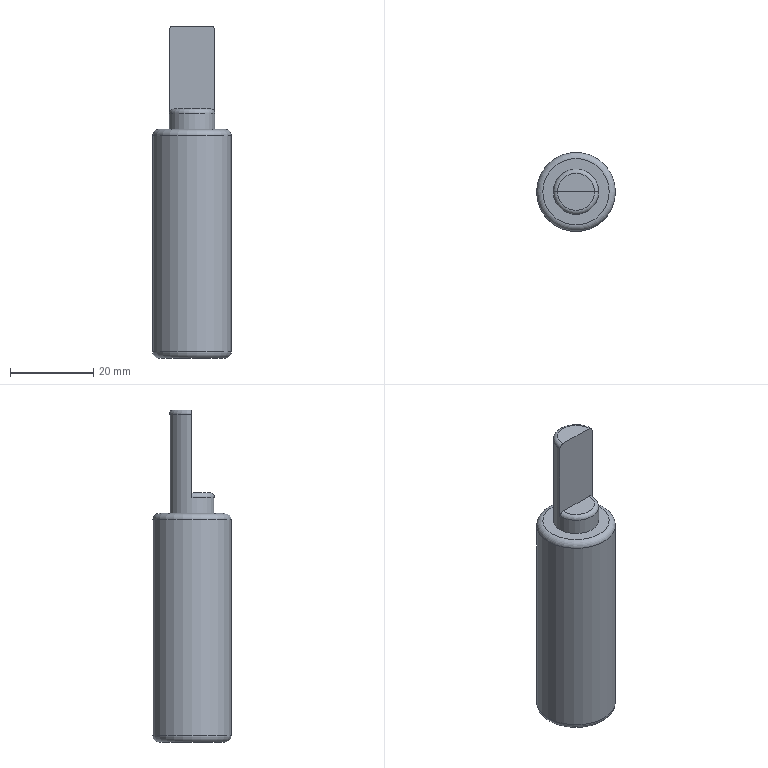Part | STEP file | 1_id1178_x_t | 1 solid | 13 faces | box 19 x 19 x 80 mm | volume 16778 mm3 | plane 5 | torus 4 | cylinder 3 | cone 1 | commonest cylinder face diameters 5.156 x1 10.922 x1 19 x1
STEP:
#1=CARTESIAN_POINT('',(0.,0.,0.));
#2=DIRECTION('',(0.,0.,1.));
#3=DIRECTION('',(1.,0.,0.));
#4=AXIS2_PLACEMENT_3D('',#1,#2,#3);
#5=CARTESIAN_POINT('',(687.464,177.5,-76.53));
#6=VERTEX_POINT('',#5);
#7=CARTESIAN_POINT('',(688.464,177.5,-75.53));
#8=VERTEX_POINT('',#7);
#9=CARTESIAN_POINT('',(687.464,177.5,-76.53));
#10=CARTESIAN_POINT('',(687.464,177.5,-76.418));
#11=CARTESIAN_POINT('',(687.483,177.5,-76.305));
#12=CARTESIAN_POINT('',(687.52,177.5,-76.199));
#13=CARTESIAN_POINT('',(687.557,177.5,-76.093));
#14=CARTESIAN_POINT('',(687.613,177.5,-75.993));
#15=CARTESIAN_POINT('',(687.683,177.5,-75.905));
#16=CARTESIAN_POINT('',(687.753,177.5,-75.818));
#17=CARTESIAN_POINT('',(687.839,177.5,-75.741));
#18=CARTESIAN_POINT('',(687.934,177.5,-75.682));
#19=CARTESIAN_POINT('',(688.029,177.5,-75.623));
#20=CARTESIAN_POINT('',(688.135,177.5,-75.579));
#21=CARTESIAN_POINT('',(688.244,177.5,-75.554));
#22=CARTESIAN_POINT('',(688.316,177.5,-75.538));
#23=CARTESIAN_POINT('',(688.39,177.5,-75.53));
#24=CARTESIAN_POINT('',(688.464,177.5,-75.53));
#25=B_SPLINE_CURVE_WITH_KNOTS('',3,(#9,#10,#11,#12,#13,#14,#15,#16,#17,#18,#19,#20,#21,#22,#23,#24),.UNSPECIFIED.,.F.,.F.,(4,3,3,3,3,4),(0.,0.2149,0.4299,0.6448,0.8598,1.),.UNSPECIFIED.);
#26=CARTESIAN_POINT('',(351.838,177.5,-123.402));
#27=DIRECTION('',(0.,1.,0.));
#28=DIRECTION('',(0.,0.,-1.));
#29=AXIS2_PLACEMENT_3D('',#26,#27,#28);
#30=PLANE('',#29);
#31=CARTESIAN_POINT('',(-46.872,-335.625));
#32=CARTESIAN_POINT('',(-46.984,-335.625));
#33=CARTESIAN_POINT('',(-47.098,-335.645));
#34=CARTESIAN_POINT('',(-47.203,-335.682));
#35=CARTESIAN_POINT('',(-47.309,-335.719));
#36=CARTESIAN_POINT('',(-47.409,-335.775));
#37=CARTESIAN_POINT('',(-47.497,-335.845));
#38=CARTESIAN_POINT('',(-47.584,-335.914));
#39=CARTESIAN_POINT('',(-47.661,-336.));
#40=CARTESIAN_POINT('',(-47.72,-336.095));
#41=CARTESIAN_POINT('',(-47.779,-336.19));
#42=CARTESIAN_POINT('',(-47.823,-336.297));
#43=CARTESIAN_POINT('',(-47.848,-336.406));
#44=CARTESIAN_POINT('',(-47.864,-336.478));
#45=CARTESIAN_POINT('',(-47.872,-336.552));
#46=CARTESIAN_POINT('',(-47.872,-336.625));
#47=B_SPLINE_CURVE_WITH_KNOTS('',3,(#31,#32,#33,#34,#35,#36,#37,#38,#39,#40,#41,#42,#43,#44,#45,#46),.UNSPECIFIED.,.F.,.F.,(4,3,3,3,3,4),(0.,0.2149,0.4299,0.6448,0.8598,1.),.UNSPECIFIED.);
#48=(GEOMETRIC_REPRESENTATION_CONTEXT(2)PARAMETRIC_REPRESENTATION_CONTEXT()REPRESENTATION_CONTEXT('',''));
#49=DEFINITIONAL_REPRESENTATION('',(#47),#48);
#50=PCURVE('',#30,#49);
#51=CARTESIAN_POINT('',(692.925,177.5,-76.53));
#52=DIRECTION('',(0.,0.,1.));
#53=DIRECTION('',(1.,0.,0.));
#54=AXIS2_PLACEMENT_3D('',#51,#52,#53);
#55=TOROIDAL_SURFACE('',#54,4.461,1.);
#56=CARTESIAN_POINT('',(3.142,0.));
#57=CARTESIAN_POINT('',(3.142,1.571));
#58=B_SPLINE_CURVE_WITH_KNOTS('',1,(#56,#57),.UNSPECIFIED.,.F.,.F.,(2,2),(0.,1.),.PIECEWISE_BEZIER_KNOTS.);
#59=(GEOMETRIC_REPRESENTATION_CONTEXT(2)PARAMETRIC_REPRESENTATION_CONTEXT()REPRESENTATION_CONTEXT('',''));
#60=DEFINITIONAL_REPRESENTATION('',(#58),#59);
#61=PCURVE('',#55,#60);
#62=SURFACE_CURVE('',#25,(#50,#61),.PCURVE_S1.);
#63=EDGE_CURVE('',#6,#8,#62,.T.);
#64=ORIENTED_EDGE('',*,*,#63,.F.);
#65=CARTESIAN_POINT('',(687.464,177.5,-56.53));
#66=VERTEX_POINT('',#65);
#67=CARTESIAN_POINT('',(687.464,177.5,-123.402));
#68=DIRECTION('',(0.,0.,1.));
#69=VECTOR('',#68,1.);
#70=LINE('',#67,#69);
#71=CARTESIAN_POINT('',(0.,-335.625));
#72=DIRECTION('',(-1.,0.));
#73=VECTOR('',#72,1.);
#74=LINE('',#71,#73);
#75=(GEOMETRIC_REPRESENTATION_CONTEXT(2)PARAMETRIC_REPRESENTATION_CONTEXT()REPRESENTATION_CONTEXT('',''));
#76=DEFINITIONAL_REPRESENTATION('',(#74),#75);
#77=PCURVE('',#30,#76);
#78=CARTESIAN_POINT('',(692.925,177.5,-142.23));
#79=DIRECTION('',(0.,0.,1.));
#80=DIRECTION('',(-1.,0.,0.));
#81=AXIS2_PLACEMENT_3D('',#78,#79,#80);
#82=CYLINDRICAL_SURFACE('',#81,5.461);
#83=CARTESIAN_POINT('',(6.283,18.828));
#84=DIRECTION('',(0.,1.));
#85=VECTOR('',#84,1.);
#86=LINE('',#83,#85);
#87=(GEOMETRIC_REPRESENTATION_CONTEXT(2)PARAMETRIC_REPRESENTATION_CONTEXT()REPRESENTATION_CONTEXT('',''));
#88=DEFINITIONAL_REPRESENTATION('',(#86),#87);
#89=PCURVE('',#82,#88);
#90=SURFACE_CURVE('',#70,(#77,#89),.PCURVE_S1.);
#91=EDGE_CURVE('',#6,#66,#90,.T.);
#92=ORIENTED_EDGE('',*,*,#91,.T.);
#93=CARTESIAN_POINT('',(688.464,177.5,-55.53));
#94=VERTEX_POINT('',#93);
#95=CARTESIAN_POINT('',(688.464,177.5,-55.53));
#96=CARTESIAN_POINT('',(688.352,177.5,-55.53));
#97=CARTESIAN_POINT('',(688.238,177.5,-55.549));
#98=CARTESIAN_POINT('',(688.133,177.5,-55.586));
#99=CARTESIAN_POINT('',(688.027,177.5,-55.623));
#100=CARTESIAN_POINT('',(687.927,177.5,-55.679));
#101=CARTESIAN_POINT('',(687.839,177.5,-55.749));
#102=CARTESIAN_POINT('',(687.752,177.5,-55.819));
#103=CARTESIAN_POINT('',(687.675,177.5,-55.905));
#104=CARTESIAN_POINT('',(687.616,177.5,-56.));
#105=CARTESIAN_POINT('',(687.557,177.5,-56.095));
#106=CARTESIAN_POINT('',(687.513,177.5,-56.201));
#107=CARTESIAN_POINT('',(687.488,177.5,-56.31));
#108=CARTESIAN_POINT('',(687.472,177.5,-56.382));
#109=CARTESIAN_POINT('',(687.464,177.5,-56.456));
#110=CARTESIAN_POINT('',(687.464,177.5,-56.53));
#111=B_SPLINE_CURVE_WITH_KNOTS('',3,(#95,#96,#97,#98,#99,#100,#101,#102,#103,#104,#105,#106,#107,#108,#109,#110),.UNSPECIFIED.,.F.,.F.,(4,3,3,3,3,4),(0.,0.2149,0.4299,0.6448,0.8598,1.),.UNSPECIFIED.);
#112=CARTESIAN_POINT('',(-67.872,-336.625));
#113=CARTESIAN_POINT('',(-67.872,-336.513));
#114=CARTESIAN_POINT('',(-67.853,-336.4));
#115=CARTESIAN_POINT('',(-67.816,-336.294));
#116=CARTESIAN_POINT('',(-67.779,-336.189));
#117=CARTESIAN_POINT('',(-67.723,-336.088));
#118=CARTESIAN_POINT('',(-67.653,-336.001));
#119=CARTESIAN_POINT('',(-67.583,-335.913));
#120=CARTESIAN_POINT('',(-67.497,-335.837));
#121=CARTESIAN_POINT('',(-67.402,-335.777));
#122=CARTESIAN_POINT('',(-67.307,-335.718));
#123=CARTESIAN_POINT('',(-67.201,-335.674));
#124=CARTESIAN_POINT('',(-67.092,-335.65));
#125=CARTESIAN_POINT('',(-67.02,-335.634));
#126=CARTESIAN_POINT('',(-66.946,-335.625));
#127=CARTESIAN_POINT('',(-66.872,-335.625));
#128=B_SPLINE_CURVE_WITH_KNOTS('',3,(#112,#113,#114,#115,#116,#117,#118,#119,#120,#121,#122,#123,#124,#125,#126,#127),.UNSPECIFIED.,.F.,.F.,(4,3,3,3,3,4),(0.,0.2149,0.4299,0.6448,0.8598,1.),.UNSPECIFIED.);
#129=(GEOMETRIC_REPRESENTATION_CONTEXT(2)PARAMETRIC_REPRESENTATION_CONTEXT()REPRESENTATION_CONTEXT('',''));
#130=DEFINITIONAL_REPRESENTATION('',(#128),#129);
#131=PCURVE('',#30,#130);
#132=CARTESIAN_POINT('',(692.925,177.5,-56.53));
#133=DIRECTION('',(0.,0.,1.));
#134=DIRECTION('',(1.,0.,0.));
#135=AXIS2_PLACEMENT_3D('',#132,#133,#134);
#136=TOROIDAL_SURFACE('',#135,4.461,1.);
#137=CARTESIAN_POINT('',(3.142,1.571));
#138=CARTESIAN_POINT('',(3.142,0.));
#139=B_SPLINE_CURVE_WITH_KNOTS('',1,(#137,#138),.UNSPECIFIED.,.F.,.F.,(2,2),(0.,1.),.PIECEWISE_BEZIER_KNOTS.);
#140=(GEOMETRIC_REPRESENTATION_CONTEXT(2)PARAMETRIC_REPRESENTATION_CONTEXT()REPRESENTATION_CONTEXT('',''));
#141=DEFINITIONAL_REPRESENTATION('',(#139),#140);
#142=PCURVE('',#136,#141);
#143=SURFACE_CURVE('',#111,(#131,#142),.PCURVE_S1.);
#144=EDGE_CURVE('',#94,#66,#143,.T.);
#145=ORIENTED_EDGE('',*,*,#144,.F.);
#146=CARTESIAN_POINT('',(697.386,177.5,-55.53));
#147=VERTEX_POINT('',#146);
#148=CARTESIAN_POINT('',(688.464,177.5,-55.53));
#149=DIRECTION('',(1.,0.000000541,0.));
#150=VECTOR('',#149,1.);
#151=LINE('',#148,#150);
#152=CARTESIAN_POINT('',(-67.872,-336.625));
#153=DIRECTION('',(0.,-1.));
#154=VECTOR('',#153,1.);
#155=LINE('',#152,#154);
#156=(GEOMETRIC_REPRESENTATION_CONTEXT(2)PARAMETRIC_REPRESENTATION_CONTEXT()REPRESENTATION_CONTEXT('',''));
#157=DEFINITIONAL_REPRESENTATION('',(#155),#156);
#158=PCURVE('',#30,#157);
#159=CARTESIAN_POINT('',(692.925,177.5,-55.53));
#160=DIRECTION('',(0.,0.,1.));
#161=DIRECTION('',(-1.,0.,0.));
#162=AXIS2_PLACEMENT_3D('',#159,#160,#161);
#163=PLANE('',#162);
#164=CARTESIAN_POINT('',(4.461,-0.00001102));
#165=DIRECTION('',(-1.,-0.000000541));
#166=VECTOR('',#165,1.);
#167=LINE('',#164,#166);
#168=(GEOMETRIC_REPRESENTATION_CONTEXT(2)PARAMETRIC_REPRESENTATION_CONTEXT()REPRESENTATION_CONTEXT('',''));
#169=DEFINITIONAL_REPRESENTATION('',(#167),#168);
#170=PCURVE('',#163,#169);
#171=SURFACE_CURVE('',#151,(#158,#170),.PCURVE_S1.);
#172=EDGE_CURVE('',#94,#147,#171,.T.);
#173=ORIENTED_EDGE('',*,*,#172,.T.);
#174=CARTESIAN_POINT('',(698.386,177.5,-56.53));
#175=VERTEX_POINT('',#174);
#176=CARTESIAN_POINT('',(697.386,177.5,-56.53));
#177=DIRECTION('',(0.000003245,-1.,0.));
#178=DIRECTION('',(1.,0.000003245,0.));
#179=AXIS2_PLACEMENT_3D('',#176,#177,#178);
#180=CIRCLE('',#179,1.);
#181=CARTESIAN_POINT('',(-66.872,-346.547));
#182=CARTESIAN_POINT('',(-68.604,-346.547));
#183=CARTESIAN_POINT('',(-67.738,-345.047));
#184=CARTESIAN_POINT('',(-66.872,-343.547));
#185=CARTESIAN_POINT('',(-66.006,-345.047));
#186=CARTESIAN_POINT('',(-65.14,-346.547));
#187=CARTESIAN_POINT('',(-66.872,-346.547));
#188=(BOUNDED_CURVE()B_SPLINE_CURVE(2,(#181,#182,#183,#184,#185,#186,#187),.UNSPECIFIED.,.T.,.F.)B_SPLINE_CURVE_WITH_KNOTS((1,2,2,2,2,1),(-2.094,0.,2.094,4.189,6.283,8.378),.UNSPECIFIED.)CURVE()GEOMETRIC_REPRESENTATION_ITEM()RATIONAL_B_SPLINE_CURVE((1.,0.5,1.,0.5,1.,0.5,1.))REPRESENTATION_ITEM(''));
#189=(GEOMETRIC_REPRESENTATION_CONTEXT(2)PARAMETRIC_REPRESENTATION_CONTEXT()REPRESENTATION_CONTEXT('',''));
#190=DEFINITIONAL_REPRESENTATION('',(#188),#189);
#191=PCURVE('',#30,#190);
#192=CARTESIAN_POINT('',(0.000003245,0.));
#193=DIRECTION('',(0.,1.));
#194=VECTOR('',#193,1.);
#195=LINE('',#192,#194);
#196=(GEOMETRIC_REPRESENTATION_CONTEXT(2)PARAMETRIC_REPRESENTATION_CONTEXT()REPRESENTATION_CONTEXT('',''));
#197=DEFINITIONAL_REPRESENTATION('',(#195),#196);
#198=PCURVE('',#136,#197);
#199=SURFACE_CURVE('',#180,(#191,#198),.PCURVE_S1.);
#200=EDGE_CURVE('',#175,#147,#199,.T.);
#201=ORIENTED_EDGE('',*,*,#200,.F.);
#202=CARTESIAN_POINT('',(698.386,177.5,-76.53));
#203=VERTEX_POINT('',#202);
#204=CARTESIAN_POINT('',(698.386,177.5,-76.53));
#205=DIRECTION('',(0.,-0.000000143,-1.));
#206=VECTOR('',#205,1.);
#207=LINE('',#204,#206);
#208=CARTESIAN_POINT('',(-46.872,-346.547));
#209=DIRECTION('',(1.,0.));
#210=VECTOR('',#209,1.);
#211=LINE('',#208,#210);
#212=(GEOMETRIC_REPRESENTATION_CONTEXT(2)PARAMETRIC_REPRESENTATION_CONTEXT()REPRESENTATION_CONTEXT('',''));
#213=DEFINITIONAL_REPRESENTATION('',(#211),#212);
#214=PCURVE('',#30,#213);
#215=CARTESIAN_POINT('',(3.142,65.7));
#216=DIRECTION('',(-0.000000026,-1.));
#217=VECTOR('',#216,1.);
#218=LINE('',#215,#217);
#219=(GEOMETRIC_REPRESENTATION_CONTEXT(2)PARAMETRIC_REPRESENTATION_CONTEXT()REPRESENTATION_CONTEXT('',''));
#220=DEFINITIONAL_REPRESENTATION('',(#218),#219);
#221=PCURVE('',#82,#220);
#222=SURFACE_CURVE('',#207,(#214,#221),.PCURVE_S1.);
#223=EDGE_CURVE('',#175,#203,#222,.T.);
#224=ORIENTED_EDGE('',*,*,#223,.T.);
#225=CARTESIAN_POINT('',(697.386,177.5,-75.53));
#226=VERTEX_POINT('',#225);
#227=CARTESIAN_POINT('',(697.386,177.5,-76.53));
#228=DIRECTION('',(-0.000003245,1.,0.));
#229=DIRECTION('',(0.,0.,1.));
#230=AXIS2_PLACEMENT_3D('',#227,#228,#229);
#231=CIRCLE('',#230,1.);
#232=CARTESIAN_POINT('',(-46.872,-345.547));
#233=DIRECTION('',(-1.,0.));
#234=AXIS2_PLACEMENT_2D('',#232,#233);
#235=CIRCLE('',#234,1.);
#236=(GEOMETRIC_REPRESENTATION_CONTEXT(2)PARAMETRIC_REPRESENTATION_CONTEXT()REPRESENTATION_CONTEXT('',''));
#237=DEFINITIONAL_REPRESENTATION('',(#235),#236);
#238=PCURVE('',#30,#237);
#239=CARTESIAN_POINT('',(6.283,1.571));
#240=DIRECTION('',(0.,-1.));
#241=VECTOR('',#240,1.);
#242=LINE('',#239,#241);
#243=(GEOMETRIC_REPRESENTATION_CONTEXT(2)PARAMETRIC_REPRESENTATION_CONTEXT()REPRESENTATION_CONTEXT('',''));
#244=DEFINITIONAL_REPRESENTATION('',(#242),#243);
#245=PCURVE('',#55,#244);
#246=SURFACE_CURVE('',#231,(#238,#245),.PCURVE_S1.);
#247=EDGE_CURVE('',#226,#203,#246,.T.);
#248=ORIENTED_EDGE('',*,*,#247,.F.);
#249=CARTESIAN_POINT('',(688.464,177.5,-75.53));
#250=DIRECTION('',(1.,0.000000541,0.));
#251=VECTOR('',#250,1.);
#252=LINE('',#249,#251);
#253=CARTESIAN_POINT('',(-47.872,-336.625));
#254=DIRECTION('',(0.,-1.));
#255=VECTOR('',#254,1.);
#256=LINE('',#253,#255);
#257=(GEOMETRIC_REPRESENTATION_CONTEXT(2)PARAMETRIC_REPRESENTATION_CONTEXT()REPRESENTATION_CONTEXT('',''));
#258=DEFINITIONAL_REPRESENTATION('',(#256),#257);
#259=PCURVE('',#30,#258);
#260=CARTESIAN_POINT('',(692.925,177.5,-75.53));
#261=DIRECTION('',(0.,0.,1.));
#262=DIRECTION('',(-1.,0.,0.));
#263=AXIS2_PLACEMENT_3D('',#260,#261,#262);
#264=PLANE('',#263);
#265=CARTESIAN_POINT('',(4.461,-0.00001102));
#266=DIRECTION('',(-1.,-0.000000541));
#267=VECTOR('',#266,1.);
#268=LINE('',#265,#267);
#269=(GEOMETRIC_REPRESENTATION_CONTEXT(2)PARAMETRIC_REPRESENTATION_CONTEXT()REPRESENTATION_CONTEXT('',''));
#270=DEFINITIONAL_REPRESENTATION('',(#268),#269);
#271=PCURVE('',#264,#270);
#272=SURFACE_CURVE('',#252,(#259,#271),.PCURVE_S1.);
#273=EDGE_CURVE('',#8,#226,#272,.T.);
#274=ORIENTED_EDGE('',*,*,#273,.F.);
#275=EDGE_LOOP('',(#64,#92,#145,#173,#201,#224,#248,#274));
#276=FACE_BOUND('',#275,.F.);
#277=ADVANCED_FACE('',(#276),#30,.F.);
#278=ORIENTED_EDGE('',*,*,#63,.F.);
#279=CARTESIAN_POINT('',(692.925,177.5,-76.53));
#280=DIRECTION('',(0.,0.,1.));
#281=DIRECTION('',(-1.,0.,0.));
#282=AXIS2_PLACEMENT_3D('',#279,#280,#281);
#283=CIRCLE('',#282,5.461);
#284=CARTESIAN_POINT('',(3.142,0.));
#285=DIRECTION('',(1.,0.));
#286=VECTOR('',#285,1.);
#287=LINE('',#284,#286);
#288=(GEOMETRIC_REPRESENTATION_CONTEXT(2)PARAMETRIC_REPRESENTATION_CONTEXT()REPRESENTATION_CONTEXT('',''));
#289=DEFINITIONAL_REPRESENTATION('',(#287),#288);
#290=PCURVE('',#55,#289);
#291=CARTESIAN_POINT('',(0.,65.7));
#292=DIRECTION('',(1.,0.));
#293=VECTOR('',#292,1.);
#294=LINE('',#291,#293);
#295=(GEOMETRIC_REPRESENTATION_CONTEXT(2)PARAMETRIC_REPRESENTATION_CONTEXT()REPRESENTATION_CONTEXT('',''));
#296=DEFINITIONAL_REPRESENTATION('',(#294),#295);
#297=PCURVE('',#82,#296);
#298=SURFACE_CURVE('',#283,(#290,#297),.PCURVE_S1.);
#299=EDGE_CURVE('',#6,#203,#298,.T.);
#300=ORIENTED_EDGE('',*,*,#299,.T.);
#301=ORIENTED_EDGE('',*,*,#247,.F.);
#302=CARTESIAN_POINT('',(692.925,177.5,-75.53));
#303=DIRECTION('',(0.,0.,1.));
#304=DIRECTION('',(-1.,0.000003705,0.));
#305=AXIS2_PLACEMENT_3D('',#302,#303,#304);
#306=CIRCLE('',#305,4.461);
#307=CARTESIAN_POINT('',(3.142,1.571));
#308=DIRECTION('',(1.,0.));
#309=VECTOR('',#308,1.);
#310=LINE('',#307,#309);
#311=(GEOMETRIC_REPRESENTATION_CONTEXT(2)PARAMETRIC_REPRESENTATION_CONTEXT()REPRESENTATION_CONTEXT('',''));
#312=DEFINITIONAL_REPRESENTATION('',(#310),#311);
#313=PCURVE('',#55,#312);
#314=CARTESIAN_POINT('',(0.,0.));
#315=DIRECTION('',(1.,-0.000003705));
#316=AXIS2_PLACEMENT_2D('',#314,#315);
#317=CIRCLE('',#316,4.461);
#318=(GEOMETRIC_REPRESENTATION_CONTEXT(2)PARAMETRIC_REPRESENTATION_CONTEXT()REPRESENTATION_CONTEXT('',''));
#319=DEFINITIONAL_REPRESENTATION('',(#317),#318);
#320=PCURVE('',#264,#319);
#321=SURFACE_CURVE('',#306,(#313,#320),.PCURVE_S1.);
#322=EDGE_CURVE('',#8,#226,#321,.T.);
#323=ORIENTED_EDGE('',*,*,#322,.F.);
#324=EDGE_LOOP('',(#278,#300,#301,#323));
#325=FACE_BOUND('',#324,.T.);
#326=ADVANCED_FACE('',(#325),#55,.T.);
#327=ORIENTED_EDGE('',*,*,#273,.F.);
#328=ORIENTED_EDGE('',*,*,#322,.T.);
#329=EDGE_LOOP('',(#327,#328));
#330=FACE_BOUND('',#329,.T.);
#331=ADVANCED_FACE('',(#330),#264,.T.);
#332=ORIENTED_EDGE('',*,*,#299,.F.);
#333=CARTESIAN_POINT('',(687.464,177.5,-80.457));
#334=VERTEX_POINT('',#333);
#335=CARTESIAN_POINT('',(687.464,177.5,-80.457));
#336=CARTESIAN_POINT('',(687.464,177.5,-76.53));
#337=B_SPLINE_CURVE_WITH_KNOTS('',1,(#335,#336),.UNSPECIFIED.,.F.,.F.,(2,2),(61.773,65.7),.PIECEWISE_BEZIER_KNOTS.);
#338=CARTESIAN_POINT('',(0.,0.));
#339=DIRECTION('',(0.,1.));
#340=VECTOR('',#339,1.);
#341=LINE('',#338,#340);
#342=(GEOMETRIC_REPRESENTATION_CONTEXT(2)PARAMETRIC_REPRESENTATION_CONTEXT()REPRESENTATION_CONTEXT('',''));
#343=DEFINITIONAL_REPRESENTATION('',(#341),#342);
#344=PCURVE('',#82,#343);
#345=CARTESIAN_POINT('',(6.283,0.));
#346=DIRECTION('',(0.,1.));
#347=VECTOR('',#346,1.);
#348=LINE('',#345,#347);
#349=(GEOMETRIC_REPRESENTATION_CONTEXT(2)PARAMETRIC_REPRESENTATION_CONTEXT()REPRESENTATION_CONTEXT('',''));
#350=DEFINITIONAL_REPRESENTATION('',(#348),#349);
#351=PCURVE('',#82,#350);
#352=SEAM_CURVE('',#337,(#344,#351),.PCURVE_S1.);
#353=EDGE_CURVE('',#334,#6,#352,.T.);
#354=ORIENTED_EDGE('',*,*,#353,.F.);
#355=CARTESIAN_POINT('',(698.386,177.5,-80.457));
#356=VERTEX_POINT('',#355);
#357=CARTESIAN_POINT('',(692.925,177.5,-80.457));
#358=DIRECTION('',(0.,0.,-1.));
#359=DIRECTION('',(1.,0.,0.));
#360=AXIS2_PLACEMENT_3D('',#357,#358,#359);
#361=CIRCLE('',#360,5.461);
#362=CARTESIAN_POINT('',(3.142,61.773));
#363=DIRECTION('',(-1.,0.));
#364=VECTOR('',#363,1.);
#365=LINE('',#362,#364);
#366=(GEOMETRIC_REPRESENTATION_CONTEXT(2)PARAMETRIC_REPRESENTATION_CONTEXT()REPRESENTATION_CONTEXT('',''));
#367=DEFINITIONAL_REPRESENTATION('',(#365),#366);
#368=PCURVE('',#82,#367);
#369=CARTESIAN_POINT('',(692.925,177.5,-80.457));
#370=DIRECTION('',(0.,0.,1.));
#371=DIRECTION('',(-1.,0.,0.));
#372=AXIS2_PLACEMENT_3D('',#369,#370,#371);
#373=PLANE('',#372);
#374=CARTESIAN_POINT('',(-5.461,0.));
#375=CARTESIAN_POINT('',(-5.461,9.459));
#376=CARTESIAN_POINT('',(2.731,4.729));
#377=CARTESIAN_POINT('',(10.922,0.));
#378=CARTESIAN_POINT('',(2.731,-4.729));
#379=CARTESIAN_POINT('',(-5.461,-9.459));
#380=CARTESIAN_POINT('',(-5.461,0.));
#381=(BOUNDED_CURVE()B_SPLINE_CURVE(2,(#374,#375,#376,#377,#378,#379,#380),.UNSPECIFIED.,.T.,.F.)B_SPLINE_CURVE_WITH_KNOTS((1,2,2,2,2,1),(-2.094,0.,2.094,4.189,6.283,8.378),.UNSPECIFIED.)CURVE()GEOMETRIC_REPRESENTATION_ITEM()RATIONAL_B_SPLINE_CURVE((1.,0.5,1.,0.5,1.,0.5,1.))REPRESENTATION_ITEM(''));
#382=(GEOMETRIC_REPRESENTATION_CONTEXT(2)PARAMETRIC_REPRESENTATION_CONTEXT()REPRESENTATION_CONTEXT('',''));
#383=DEFINITIONAL_REPRESENTATION('',(#381),#382);
#384=PCURVE('',#373,#383);
#385=SURFACE_CURVE('',#361,(#368,#384),.PCURVE_S1.);
#386=EDGE_CURVE('',#356,#334,#385,.T.);
#387=ORIENTED_EDGE('',*,*,#386,.F.);
#388=CARTESIAN_POINT('',(692.925,177.5,-80.457));
#389=DIRECTION('',(0.,0.,-1.));
#390=DIRECTION('',(1.,0.,0.));
#391=AXIS2_PLACEMENT_3D('',#388,#389,#390);
#392=CIRCLE('',#391,5.461);
#393=CARTESIAN_POINT('',(9.425,61.773));
#394=DIRECTION('',(-1.,0.));
#395=VECTOR('',#394,1.);
#396=LINE('',#393,#395);
#397=(GEOMETRIC_REPRESENTATION_CONTEXT(2)PARAMETRIC_REPRESENTATION_CONTEXT()REPRESENTATION_CONTEXT('',''));
#398=DEFINITIONAL_REPRESENTATION('',(#396),#397);
#399=PCURVE('',#82,#398);
#400=CARTESIAN_POINT('',(-5.461,0.));
#401=CARTESIAN_POINT('',(-5.461,9.459));
#402=CARTESIAN_POINT('',(2.731,4.729));
#403=CARTESIAN_POINT('',(10.922,0.));
#404=CARTESIAN_POINT('',(2.731,-4.729));
#405=CARTESIAN_POINT('',(-5.461,-9.459));
#406=CARTESIAN_POINT('',(-5.461,0.));
#407=(BOUNDED_CURVE()B_SPLINE_CURVE(2,(#400,#401,#402,#403,#404,#405,#406),.UNSPECIFIED.,.T.,.F.)B_SPLINE_CURVE_WITH_KNOTS((1,2,2,2,2,1),(-2.094,0.,2.094,4.189,6.283,8.378),.UNSPECIFIED.)CURVE()GEOMETRIC_REPRESENTATION_ITEM()RATIONAL_B_SPLINE_CURVE((1.,0.5,1.,0.5,1.,0.5,1.))REPRESENTATION_ITEM(''));
#408=(GEOMETRIC_REPRESENTATION_CONTEXT(2)PARAMETRIC_REPRESENTATION_CONTEXT()REPRESENTATION_CONTEXT('',''));
#409=DEFINITIONAL_REPRESENTATION('',(#407),#408);
#410=PCURVE('',#373,#409);
#411=SURFACE_CURVE('',#392,(#399,#410),.PCURVE_S1.);
#412=EDGE_CURVE('',#334,#356,#411,.T.);
#413=ORIENTED_EDGE('',*,*,#412,.F.);
#414=ORIENTED_EDGE('',*,*,#353,.T.);
#415=ORIENTED_EDGE('',*,*,#91,.T.);
#416=CARTESIAN_POINT('',(692.925,177.5,-56.53));
#417=DIRECTION('',(0.,0.,1.));
#418=DIRECTION('',(1.,0.,0.));
#419=AXIS2_PLACEMENT_3D('',#416,#417,#418);
#420=CIRCLE('',#419,5.461);
#421=CARTESIAN_POINT('',(3.142,85.7));
#422=DIRECTION('',(1.,0.));
#423=VECTOR('',#422,1.);
#424=LINE('',#421,#423);
#425=(GEOMETRIC_REPRESENTATION_CONTEXT(2)PARAMETRIC_REPRESENTATION_CONTEXT()REPRESENTATION_CONTEXT('',''));
#426=DEFINITIONAL_REPRESENTATION('',(#424),#425);
#427=PCURVE('',#82,#426);
#428=CARTESIAN_POINT('',(0.,0.));
#429=DIRECTION('',(1.,0.));
#430=VECTOR('',#429,1.);
#431=LINE('',#428,#430);
#432=(GEOMETRIC_REPRESENTATION_CONTEXT(2)PARAMETRIC_REPRESENTATION_CONTEXT()REPRESENTATION_CONTEXT('',''));
#433=DEFINITIONAL_REPRESENTATION('',(#431),#432);
#434=PCURVE('',#136,#433);
#435=SURFACE_CURVE('',#420,(#427,#434),.PCURVE_S1.);
#436=EDGE_CURVE('',#175,#66,#435,.T.);
#437=ORIENTED_EDGE('',*,*,#436,.F.);
#438=ORIENTED_EDGE('',*,*,#223,.T.);
#439=EDGE_LOOP('',(#332,#354,#387,#413,#414,#415,#437,#438));
#440=FACE_BOUND('',#439,.T.);
#441=ADVANCED_FACE('',(#440),#82,.T.);
#442=CARTESIAN_POINT('',(684.925,177.5,-80.457));
#443=VERTEX_POINT('',#442);
#444=CARTESIAN_POINT('',(700.925,177.5,-80.457));
#445=VERTEX_POINT('',#444);
#446=CARTESIAN_POINT('',(692.925,177.5,-80.457));
#447=DIRECTION('',(0.,0.,1.));
#448=DIRECTION('',(-1.,0.,0.));
#449=AXIS2_PLACEMENT_3D('',#446,#447,#448);
#450=CIRCLE('',#449,8.);
#451=CARTESIAN_POINT('',(0.,0.));
#452=DIRECTION('',(1.,0.));
#453=AXIS2_PLACEMENT_2D('',#451,#452);
#454=CIRCLE('',#453,8.);
#455=(GEOMETRIC_REPRESENTATION_CONTEXT(2)PARAMETRIC_REPRESENTATION_CONTEXT()REPRESENTATION_CONTEXT('',''));
#456=DEFINITIONAL_REPRESENTATION('',(#454),#455);
#457=PCURVE('',#373,#456);
#458=CARTESIAN_POINT('',(692.925,177.5,-81.957));
#459=DIRECTION('',(0.,0.,1.));
#460=DIRECTION('',(1.,0.,0.));
#461=AXIS2_PLACEMENT_3D('',#458,#459,#460);
#462=TOROIDAL_SURFACE('',#461,8.,1.5);
#463=CARTESIAN_POINT('',(3.142,7.854));
#464=DIRECTION('',(1.,0.));
#465=VECTOR('',#464,1.);
#466=LINE('',#463,#465);
#467=(GEOMETRIC_REPRESENTATION_CONTEXT(2)PARAMETRIC_REPRESENTATION_CONTEXT()REPRESENTATION_CONTEXT('',''));
#468=DEFINITIONAL_REPRESENTATION('',(#466),#467);
#469=PCURVE('',#462,#468);
#470=SURFACE_CURVE('',#450,(#457,#469),.PCURVE_S1.);
#471=EDGE_CURVE('',#443,#445,#470,.T.);
#472=ORIENTED_EDGE('',*,*,#471,.T.);
#473=CARTESIAN_POINT('',(692.925,177.5,-80.457));
#474=DIRECTION('',(0.,0.,1.));
#475=DIRECTION('',(-1.,0.,0.));
#476=AXIS2_PLACEMENT_3D('',#473,#474,#475);
#477=CIRCLE('',#476,8.);
#478=CARTESIAN_POINT('',(0.,0.));
#479=DIRECTION('',(1.,0.));
#480=AXIS2_PLACEMENT_2D('',#478,#479);
#481=CIRCLE('',#480,8.);
#482=(GEOMETRIC_REPRESENTATION_CONTEXT(2)PARAMETRIC_REPRESENTATION_CONTEXT()REPRESENTATION_CONTEXT('',''));
#483=DEFINITIONAL_REPRESENTATION('',(#481),#482);
#484=PCURVE('',#373,#483);
#485=CARTESIAN_POINT('',(-3.142,7.854));
#486=DIRECTION('',(1.,0.));
#487=VECTOR('',#486,1.);
#488=LINE('',#485,#487);
#489=(GEOMETRIC_REPRESENTATION_CONTEXT(2)PARAMETRIC_REPRESENTATION_CONTEXT()REPRESENTATION_CONTEXT('',''));
#490=DEFINITIONAL_REPRESENTATION('',(#488),#489);
#491=PCURVE('',#462,#490);
#492=SURFACE_CURVE('',#477,(#484,#491),.PCURVE_S1.);
#493=EDGE_CURVE('',#445,#443,#492,.T.);
#494=ORIENTED_EDGE('',*,*,#493,.T.);
#495=EDGE_LOOP('',(#472,#494));
#496=FACE_BOUND('',#495,.T.);
#497=ORIENTED_EDGE('',*,*,#386,.T.);
#498=ORIENTED_EDGE('',*,*,#412,.T.);
#499=EDGE_LOOP('',(#497,#498));
#500=FACE_BOUND('',#499,.T.);
#501=ADVANCED_FACE('',(#496,#500),#373,.T.);
#502=ORIENTED_EDGE('',*,*,#493,.F.);
#503=CARTESIAN_POINT('',(702.425,177.5,-81.957));
#504=VERTEX_POINT('',#503);
#505=CARTESIAN_POINT('',(702.425,177.5,-81.957));
#506=CARTESIAN_POINT('',(702.425,177.5,-81.556));
#507=CARTESIAN_POINT('',(702.297,177.5,-81.166));
#508=CARTESIAN_POINT('',(702.053,177.5,-80.829));
#509=CARTESIAN_POINT('',(701.716,177.5,-80.585));
#510=CARTESIAN_POINT('',(701.326,177.5,-80.457));
#511=CARTESIAN_POINT('',(700.925,177.5,-80.457));
#512=(BOUNDED_CURVE()B_SPLINE_CURVE(6,(#505,#506,#507,#508,#509,#510,#511),.UNSPECIFIED.,.F.,.F.)B_SPLINE_CURVE_WITH_KNOTS((7,7),(0.,1.571),.PIECEWISE_BEZIER_KNOTS.)CURVE()GEOMETRIC_REPRESENTATION_ITEM()RATIONAL_B_SPLINE_CURVE((1.031,1.01,0.9979,0.994,0.9979,1.01,1.031))REPRESENTATION_ITEM(''));
#513=CARTESIAN_POINT('',(0.,6.283));
#514=DIRECTION('',(0.,1.));
#515=VECTOR('',#514,1.);
#516=LINE('',#513,#515);
#517=(GEOMETRIC_REPRESENTATION_CONTEXT(2)PARAMETRIC_REPRESENTATION_CONTEXT()REPRESENTATION_CONTEXT('',''));
#518=DEFINITIONAL_REPRESENTATION('',(#516),#517);
#519=PCURVE('',#462,#518);
#520=CARTESIAN_POINT('',(6.283,6.283));
#521=DIRECTION('',(0.,1.));
#522=VECTOR('',#521,1.);
#523=LINE('',#520,#522);
#524=(GEOMETRIC_REPRESENTATION_CONTEXT(2)PARAMETRIC_REPRESENTATION_CONTEXT()REPRESENTATION_CONTEXT('',''));
#525=DEFINITIONAL_REPRESENTATION('',(#523),#524);
#526=PCURVE('',#462,#525);
#527=SEAM_CURVE('',#512,(#519,#526),.PCURVE_S1.);
#528=EDGE_CURVE('',#504,#445,#527,.T.);
#529=ORIENTED_EDGE('',*,*,#528,.F.);
#530=CARTESIAN_POINT('',(683.425,177.5,-81.957));
#531=VERTEX_POINT('',#530);
#532=CARTESIAN_POINT('',(692.925,177.5,-81.957));
#533=DIRECTION('',(0.,0.,1.));
#534=DIRECTION('',(1.,0.,0.));
#535=AXIS2_PLACEMENT_3D('',#532,#533,#534);
#536=CIRCLE('',#535,9.5);
#537=CARTESIAN_POINT('',(0.,6.283));
#538=DIRECTION('',(1.,0.));
#539=VECTOR('',#538,1.);
#540=LINE('',#537,#539);
#541=(GEOMETRIC_REPRESENTATION_CONTEXT(2)PARAMETRIC_REPRESENTATION_CONTEXT()REPRESENTATION_CONTEXT('',''));
#542=DEFINITIONAL_REPRESENTATION('',(#540),#541);
#543=PCURVE('',#462,#542);
#544=CARTESIAN_POINT('',(692.925,177.5,-135.53));
#545=DIRECTION('',(0.,0.,1.));
#546=DIRECTION('',(-1.,0.,0.));
#547=AXIS2_PLACEMENT_3D('',#544,#545,#546);
#548=CYLINDRICAL_SURFACE('',#547,9.5);
#549=CARTESIAN_POINT('',(3.142,53.573));
#550=DIRECTION('',(1.,0.));
#551=VECTOR('',#550,1.);
#552=LINE('',#549,#551);
#553=(GEOMETRIC_REPRESENTATION_CONTEXT(2)PARAMETRIC_REPRESENTATION_CONTEXT()REPRESENTATION_CONTEXT('',''));
#554=DEFINITIONAL_REPRESENTATION('',(#552),#553);
#555=PCURVE('',#548,#554);
#556=SURFACE_CURVE('',#536,(#543,#555),.PCURVE_S1.);
#557=EDGE_CURVE('',#504,#531,#556,.T.);
#558=ORIENTED_EDGE('',*,*,#557,.T.);
#559=CARTESIAN_POINT('',(692.925,177.5,-81.957));
#560=DIRECTION('',(0.,0.,1.));
#561=DIRECTION('',(1.,0.,0.));
#562=AXIS2_PLACEMENT_3D('',#559,#560,#561);
#563=CIRCLE('',#562,9.5);
#564=CARTESIAN_POINT('',(0.,6.283));
#565=DIRECTION('',(1.,0.));
#566=VECTOR('',#565,1.);
#567=LINE('',#564,#566);
#568=(GEOMETRIC_REPRESENTATION_CONTEXT(2)PARAMETRIC_REPRESENTATION_CONTEXT()REPRESENTATION_CONTEXT('',''));
#569=DEFINITIONAL_REPRESENTATION('',(#567),#568);
#570=PCURVE('',#462,#569);
#571=CARTESIAN_POINT('',(-3.142,53.573));
#572=DIRECTION('',(1.,0.));
#573=VECTOR('',#572,1.);
#574=LINE('',#571,#573);
#575=(GEOMETRIC_REPRESENTATION_CONTEXT(2)PARAMETRIC_REPRESENTATION_CONTEXT()REPRESENTATION_CONTEXT('',''));
#576=DEFINITIONAL_REPRESENTATION('',(#574),#575);
#577=PCURVE('',#548,#576);
#578=SURFACE_CURVE('',#563,(#570,#577),.PCURVE_S1.);
#579=EDGE_CURVE('',#531,#504,#578,.T.);
#580=ORIENTED_EDGE('',*,*,#579,.T.);
#581=ORIENTED_EDGE('',*,*,#528,.T.);
#582=ORIENTED_EDGE('',*,*,#471,.F.);
#583=EDGE_LOOP('',(#502,#529,#558,#580,#581,#582));
#584=FACE_BOUND('',#583,.T.);
#585=ADVANCED_FACE('',(#584),#462,.T.);
#586=ORIENTED_EDGE('',*,*,#579,.F.);
#587=CARTESIAN_POINT('',(683.425,177.5,-134.03));
#588=VERTEX_POINT('',#587);
#589=CARTESIAN_POINT('',(683.425,177.5,-134.03));
#590=CARTESIAN_POINT('',(683.425,177.5,-81.957));
#591=B_SPLINE_CURVE_WITH_KNOTS('',1,(#589,#590),.UNSPECIFIED.,.F.,.F.,(2,2),(1.5,53.573),.PIECEWISE_BEZIER_KNOTS.);
#592=CARTESIAN_POINT('',(0.,0.));
#593=DIRECTION('',(0.,1.));
#594=VECTOR('',#593,1.);
#595=LINE('',#592,#594);
#596=(GEOMETRIC_REPRESENTATION_CONTEXT(2)PARAMETRIC_REPRESENTATION_CONTEXT()REPRESENTATION_CONTEXT('',''));
#597=DEFINITIONAL_REPRESENTATION('',(#595),#596);
#598=PCURVE('',#548,#597);
#599=CARTESIAN_POINT('',(6.283,0.));
#600=DIRECTION('',(0.,1.));
#601=VECTOR('',#600,1.);
#602=LINE('',#599,#601);
#603=(GEOMETRIC_REPRESENTATION_CONTEXT(2)PARAMETRIC_REPRESENTATION_CONTEXT()REPRESENTATION_CONTEXT('',''));
#604=DEFINITIONAL_REPRESENTATION('',(#602),#603);
#605=PCURVE('',#548,#604);
#606=SEAM_CURVE('',#591,(#598,#605),.PCURVE_S1.);
#607=EDGE_CURVE('',#588,#531,#606,.T.);
#608=ORIENTED_EDGE('',*,*,#607,.F.);
#609=CARTESIAN_POINT('',(692.925,177.5,-134.03));
#610=DIRECTION('',(0.,0.,-1.));
#611=DIRECTION('',(-1.,0.,0.));
#612=AXIS2_PLACEMENT_3D('',#609,#610,#611);
#613=CIRCLE('',#612,9.5);
#614=CARTESIAN_POINT('',(6.283,1.5));
#615=DIRECTION('',(-1.,0.));
#616=VECTOR('',#615,1.);
#617=LINE('',#614,#616);
#618=(GEOMETRIC_REPRESENTATION_CONTEXT(2)PARAMETRIC_REPRESENTATION_CONTEXT()REPRESENTATION_CONTEXT('',''));
#619=DEFINITIONAL_REPRESENTATION('',(#617),#618);
#620=PCURVE('',#548,#619);
#621=CARTESIAN_POINT('',(692.925,177.5,-134.03));
#622=DIRECTION('',(0.,0.,-1.));
#623=DIRECTION('',(-1.,0.,0.));
#624=AXIS2_PLACEMENT_3D('',#621,#622,#623);
#625=TOROIDAL_SURFACE('',#624,8.,1.5);
#626=CARTESIAN_POINT('',(0.,6.283));
#627=DIRECTION('',(1.,0.));
#628=VECTOR('',#627,1.);
#629=LINE('',#626,#628);
#630=(GEOMETRIC_REPRESENTATION_CONTEXT(2)PARAMETRIC_REPRESENTATION_CONTEXT()REPRESENTATION_CONTEXT('',''));
#631=DEFINITIONAL_REPRESENTATION('',(#629),#630);
#632=PCURVE('',#625,#631);
#633=SURFACE_CURVE('',#613,(#620,#632),.PCURVE_S1.);
#634=EDGE_CURVE('',#588,#588,#633,.T.);
#635=ORIENTED_EDGE('',*,*,#634,.F.);
#636=ORIENTED_EDGE('',*,*,#607,.T.);
#637=ORIENTED_EDGE('',*,*,#557,.F.);
#638=EDGE_LOOP('',(#586,#608,#635,#636,#637));
#639=FACE_BOUND('',#638,.T.);
#640=ADVANCED_FACE('',(#639),#548,.T.);
#641=CARTESIAN_POINT('',(684.925,177.5,-135.53));
#642=VERTEX_POINT('',#641);
#643=CARTESIAN_POINT('',(700.925,177.5,-135.53));
#644=VERTEX_POINT('',#643);
#645=CARTESIAN_POINT('',(692.925,177.5,-135.53));
#646=DIRECTION('',(0.,0.,-1.));
#647=DIRECTION('',(1.,0.,0.));
#648=AXIS2_PLACEMENT_3D('',#645,#646,#647);
#649=CIRCLE('',#648,8.);
#650=CARTESIAN_POINT('',(-3.142,7.854));
#651=DIRECTION('',(1.,0.));
#652=VECTOR('',#651,1.);
#653=LINE('',#650,#652);
#654=(GEOMETRIC_REPRESENTATION_CONTEXT(2)PARAMETRIC_REPRESENTATION_CONTEXT()REPRESENTATION_CONTEXT('',''));
#655=DEFINITIONAL_REPRESENTATION('',(#653),#654);
#656=PCURVE('',#625,#655);
#657=CARTESIAN_POINT('',(692.925,177.5,-135.53));
#658=DIRECTION('',(0.,0.,-1.));
#659=DIRECTION('',(1.,0.,0.));
#660=AXIS2_PLACEMENT_3D('',#657,#658,#659);
#661=PLANE('',#660);
#662=CARTESIAN_POINT('',(0.,0.));
#663=DIRECTION('',(1.,0.));
#664=AXIS2_PLACEMENT_2D('',#662,#663);
#665=CIRCLE('',#664,8.);
#666=(GEOMETRIC_REPRESENTATION_CONTEXT(2)PARAMETRIC_REPRESENTATION_CONTEXT()REPRESENTATION_CONTEXT('',''));
#667=DEFINITIONAL_REPRESENTATION('',(#665),#666);
#668=PCURVE('',#661,#667);
#669=SURFACE_CURVE('',#649,(#656,#668),.PCURVE_S1.);
#670=EDGE_CURVE('',#642,#644,#669,.T.);
#671=ORIENTED_EDGE('',*,*,#670,.F.);
#672=CARTESIAN_POINT('',(683.425,177.5,-134.03));
#673=CARTESIAN_POINT('',(683.425,177.5,-134.431));
#674=CARTESIAN_POINT('',(683.552,177.5,-134.822));
#675=CARTESIAN_POINT('',(683.797,177.5,-135.158));
#676=CARTESIAN_POINT('',(684.133,177.5,-135.402));
#677=CARTESIAN_POINT('',(684.524,177.5,-135.53));
#678=CARTESIAN_POINT('',(684.925,177.5,-135.53));
#679=(BOUNDED_CURVE()B_SPLINE_CURVE(6,(#672,#673,#674,#675,#676,#677,#678),.UNSPECIFIED.,.F.,.F.)B_SPLINE_CURVE_WITH_KNOTS((7,7),(0.,1.571),.PIECEWISE_BEZIER_KNOTS.)CURVE()GEOMETRIC_REPRESENTATION_ITEM()RATIONAL_B_SPLINE_CURVE((1.031,1.01,0.9979,0.994,0.9979,1.01,1.031))REPRESENTATION_ITEM(''));
#680=CARTESIAN_POINT('',(0.,6.283));
#681=DIRECTION('',(0.,1.));
#682=VECTOR('',#681,1.);
#683=LINE('',#680,#682);
#684=(GEOMETRIC_REPRESENTATION_CONTEXT(2)PARAMETRIC_REPRESENTATION_CONTEXT()REPRESENTATION_CONTEXT('',''));
#685=DEFINITIONAL_REPRESENTATION('',(#683),#684);
#686=PCURVE('',#625,#685);
#687=CARTESIAN_POINT('',(6.283,6.283));
#688=DIRECTION('',(0.,1.));
#689=VECTOR('',#688,1.);
#690=LINE('',#687,#689);
#691=(GEOMETRIC_REPRESENTATION_CONTEXT(2)PARAMETRIC_REPRESENTATION_CONTEXT()REPRESENTATION_CONTEXT('',''));
#692=DEFINITIONAL_REPRESENTATION('',(#690),#691);
#693=PCURVE('',#625,#692);
#694=SEAM_CURVE('',#679,(#686,#693),.PCURVE_S1.);
#695=EDGE_CURVE('',#588,#642,#694,.T.);
#696=ORIENTED_EDGE('',*,*,#695,.F.);
#697=ORIENTED_EDGE('',*,*,#634,.T.);
#698=ORIENTED_EDGE('',*,*,#695,.T.);
#699=CARTESIAN_POINT('',(692.925,177.5,-135.53));
#700=DIRECTION('',(0.,0.,-1.));
#701=DIRECTION('',(1.,0.,0.));
#702=AXIS2_PLACEMENT_3D('',#699,#700,#701);
#703=CIRCLE('',#702,8.);
#704=CARTESIAN_POINT('',(3.142,7.854));
#705=DIRECTION('',(1.,0.));
#706=VECTOR('',#705,1.);
#707=LINE('',#704,#706);
#708=(GEOMETRIC_REPRESENTATION_CONTEXT(2)PARAMETRIC_REPRESENTATION_CONTEXT()REPRESENTATION_CONTEXT('',''));
#709=DEFINITIONAL_REPRESENTATION('',(#707),#708);
#710=PCURVE('',#625,#709);
#711=CARTESIAN_POINT('',(0.,0.));
#712=DIRECTION('',(1.,0.));
#713=AXIS2_PLACEMENT_2D('',#711,#712);
#714=CIRCLE('',#713,8.);
#715=(GEOMETRIC_REPRESENTATION_CONTEXT(2)PARAMETRIC_REPRESENTATION_CONTEXT()REPRESENTATION_CONTEXT('',''));
#716=DEFINITIONAL_REPRESENTATION('',(#714),#715);
#717=PCURVE('',#661,#716);
#718=SURFACE_CURVE('',#703,(#710,#717),.PCURVE_S1.);
#719=EDGE_CURVE('',#644,#642,#718,.T.);
#720=ORIENTED_EDGE('',*,*,#719,.F.);
#721=EDGE_LOOP('',(#671,#696,#697,#698,#720));
#722=FACE_BOUND('',#721,.T.);
#723=ADVANCED_FACE('',(#722),#625,.T.);
#724=ORIENTED_EDGE('',*,*,#719,.T.);
#725=ORIENTED_EDGE('',*,*,#670,.T.);
#726=EDGE_LOOP('',(#724,#725));
#727=FACE_BOUND('',#726,.T.);
#728=CARTESIAN_POINT('',(695.503,177.5,-135.53));
#729=VERTEX_POINT('',#728);
#730=CARTESIAN_POINT('',(690.347,177.5,-135.53));
#731=VERTEX_POINT('',#730);
#732=CARTESIAN_POINT('',(692.925,177.5,-135.53));
#733=DIRECTION('',(0.,0.,1.));
#734=DIRECTION('',(1.,0.,0.));
#735=AXIS2_PLACEMENT_3D('',#732,#733,#734);
#736=CIRCLE('',#735,2.578);
#737=CARTESIAN_POINT('',(2.578,0.));
#738=CARTESIAN_POINT('',(2.578,-4.465));
#739=CARTESIAN_POINT('',(-1.289,-2.233));
#740=CARTESIAN_POINT('',(-5.156,0.));
#741=CARTESIAN_POINT('',(-1.289,2.233));
#742=CARTESIAN_POINT('',(2.578,4.465));
#743=CARTESIAN_POINT('',(2.578,0.));
#744=(BOUNDED_CURVE()B_SPLINE_CURVE(2,(#737,#738,#739,#740,#741,#742,#743),.UNSPECIFIED.,.T.,.F.)B_SPLINE_CURVE_WITH_KNOTS((1,2,2,2,2,1),(-2.094,0.,2.094,4.189,6.283,8.378),.UNSPECIFIED.)CURVE()GEOMETRIC_REPRESENTATION_ITEM()RATIONAL_B_SPLINE_CURVE((1.,0.5,1.,0.5,1.,0.5,1.))REPRESENTATION_ITEM(''));
#745=(GEOMETRIC_REPRESENTATION_CONTEXT(2)PARAMETRIC_REPRESENTATION_CONTEXT()REPRESENTATION_CONTEXT('',''));
#746=DEFINITIONAL_REPRESENTATION('',(#744),#745);
#747=PCURVE('',#661,#746);
#748=CARTESIAN_POINT('',(692.925,177.5,-135.53));
#749=DIRECTION('',(0.,0.,1.));
#750=DIRECTION('',(-1.,0.,0.));
#751=AXIS2_PLACEMENT_3D('',#748,#749,#750);
#752=CYLINDRICAL_SURFACE('',#751,2.578);
#753=CARTESIAN_POINT('',(3.142,0.));
#754=DIRECTION('',(1.,0.));
#755=VECTOR('',#754,1.);
#756=LINE('',#753,#755);
#757=(GEOMETRIC_REPRESENTATION_CONTEXT(2)PARAMETRIC_REPRESENTATION_CONTEXT()REPRESENTATION_CONTEXT('',''));
#758=DEFINITIONAL_REPRESENTATION('',(#756),#757);
#759=PCURVE('',#752,#758);
#760=SURFACE_CURVE('',#736,(#747,#759),.PCURVE_S1.);
#761=EDGE_CURVE('',#729,#731,#760,.T.);
#762=ORIENTED_EDGE('',*,*,#761,.T.);
#763=CARTESIAN_POINT('',(692.925,177.5,-135.53));
#764=DIRECTION('',(0.,0.,1.));
#765=DIRECTION('',(1.,0.,0.));
#766=AXIS2_PLACEMENT_3D('',#763,#764,#765);
#767=CIRCLE('',#766,2.578);
#768=CARTESIAN_POINT('',(2.578,0.));
#769=CARTESIAN_POINT('',(2.578,-4.465));
#770=CARTESIAN_POINT('',(-1.289,-2.233));
#771=CARTESIAN_POINT('',(-5.156,0.));
#772=CARTESIAN_POINT('',(-1.289,2.233));
#773=CARTESIAN_POINT('',(2.578,4.465));
#774=CARTESIAN_POINT('',(2.578,0.));
#775=(BOUNDED_CURVE()B_SPLINE_CURVE(2,(#768,#769,#770,#771,#772,#773,#774),.UNSPECIFIED.,.T.,.F.)B_SPLINE_CURVE_WITH_KNOTS((1,2,2,2,2,1),(-2.094,0.,2.094,4.189,6.283,8.378),.UNSPECIFIED.)CURVE()GEOMETRIC_REPRESENTATION_ITEM()RATIONAL_B_SPLINE_CURVE((1.,0.5,1.,0.5,1.,0.5,1.))REPRESENTATION_ITEM(''));
#776=(GEOMETRIC_REPRESENTATION_CONTEXT(2)PARAMETRIC_REPRESENTATION_CONTEXT()REPRESENTATION_CONTEXT('',''));
#777=DEFINITIONAL_REPRESENTATION('',(#775),#776);
#778=PCURVE('',#661,#777);
#779=CARTESIAN_POINT('',(-3.142,0.));
#780=DIRECTION('',(1.,0.));
#781=VECTOR('',#780,1.);
#782=LINE('',#779,#781);
#783=(GEOMETRIC_REPRESENTATION_CONTEXT(2)PARAMETRIC_REPRESENTATION_CONTEXT()REPRESENTATION_CONTEXT('',''));
#784=DEFINITIONAL_REPRESENTATION('',(#782),#783);
#785=PCURVE('',#752,#784);
#786=SURFACE_CURVE('',#767,(#778,#785),.PCURVE_S1.);
#787=EDGE_CURVE('',#731,#729,#786,.T.);
#788=ORIENTED_EDGE('',*,*,#787,.T.);
#789=EDGE_LOOP('',(#762,#788));
#790=FACE_BOUND('',#789,.T.);
#791=ADVANCED_FACE('',(#727,#790),#661,.T.);
#792=CARTESIAN_POINT('',(690.347,177.5,-127.796));
#793=VERTEX_POINT('',#792);
#794=CARTESIAN_POINT('',(695.503,177.5,-127.796));
#795=VERTEX_POINT('',#794);
#796=CARTESIAN_POINT('',(692.925,177.5,-127.796));
#797=DIRECTION('',(0.,0.,-1.));
#798=DIRECTION('',(-1.,0.,0.));
#799=AXIS2_PLACEMENT_3D('',#796,#797,#798);
#800=CIRCLE('',#799,2.578);
#801=CARTESIAN_POINT('',(6.283,7.734));
#802=DIRECTION('',(-1.,0.));
#803=VECTOR('',#802,1.);
#804=LINE('',#801,#803);
#805=(GEOMETRIC_REPRESENTATION_CONTEXT(2)PARAMETRIC_REPRESENTATION_CONTEXT()REPRESENTATION_CONTEXT('',''));
#806=DEFINITIONAL_REPRESENTATION('',(#804),#805);
#807=PCURVE('',#752,#806);
#808=CARTESIAN_POINT('',(692.925,177.5,-127.047));
#809=DIRECTION('',(0.,0.,-1.));
#810=DIRECTION('',(1.,0.,0.));
#811=AXIS2_PLACEMENT_3D('',#808,#809,#810);
#812=CONICAL_SURFACE('',#811,1.332,1.03);
#813=CARTESIAN_POINT('',(3.142,0.7485));
#814=DIRECTION('',(1.,0.));
#815=VECTOR('',#814,1.);
#816=LINE('',#813,#815);
#817=(GEOMETRIC_REPRESENTATION_CONTEXT(2)PARAMETRIC_REPRESENTATION_CONTEXT()REPRESENTATION_CONTEXT('',''));
#818=DEFINITIONAL_REPRESENTATION('',(#816),#817);
#819=PCURVE('',#812,#818);
#820=SURFACE_CURVE('',#800,(#807,#819),.PCURVE_S1.);
#821=EDGE_CURVE('',#793,#795,#820,.T.);
#822=ORIENTED_EDGE('',*,*,#821,.T.);
#823=CARTESIAN_POINT('',(692.925,177.5,-127.796));
#824=DIRECTION('',(0.,0.,-1.));
#825=DIRECTION('',(-1.,0.,0.));
#826=AXIS2_PLACEMENT_3D('',#823,#824,#825);
#827=CIRCLE('',#826,2.578);
#828=CARTESIAN_POINT('',(6.283,7.734));
#829=DIRECTION('',(-1.,0.));
#830=VECTOR('',#829,1.);
#831=LINE('',#828,#830);
#832=(GEOMETRIC_REPRESENTATION_CONTEXT(2)PARAMETRIC_REPRESENTATION_CONTEXT()REPRESENTATION_CONTEXT('',''));
#833=DEFINITIONAL_REPRESENTATION('',(#831),#832);
#834=PCURVE('',#752,#833);
#835=CARTESIAN_POINT('',(-3.142,0.7485));
#836=DIRECTION('',(1.,0.));
#837=VECTOR('',#836,1.);
#838=LINE('',#835,#837);
#839=(GEOMETRIC_REPRESENTATION_CONTEXT(2)PARAMETRIC_REPRESENTATION_CONTEXT()REPRESENTATION_CONTEXT('',''));
#840=DEFINITIONAL_REPRESENTATION('',(#838),#839);
#841=PCURVE('',#812,#840);
#842=SURFACE_CURVE('',#827,(#834,#841),.PCURVE_S1.);
#843=EDGE_CURVE('',#795,#793,#842,.T.);
#844=ORIENTED_EDGE('',*,*,#843,.T.);
#845=CARTESIAN_POINT('',(690.347,177.5,-135.53));
#846=CARTESIAN_POINT('',(690.347,177.5,-127.796));
#847=B_SPLINE_CURVE_WITH_KNOTS('',1,(#845,#846),.UNSPECIFIED.,.F.,.F.,(2,2),(0.,7.734),.PIECEWISE_BEZIER_KNOTS.);
#848=CARTESIAN_POINT('',(0.,0.));
#849=DIRECTION('',(0.,1.));
#850=VECTOR('',#849,1.);
#851=LINE('',#848,#850);
#852=(GEOMETRIC_REPRESENTATION_CONTEXT(2)PARAMETRIC_REPRESENTATION_CONTEXT()REPRESENTATION_CONTEXT('',''));
#853=DEFINITIONAL_REPRESENTATION('',(#851),#852);
#854=PCURVE('',#752,#853);
#855=CARTESIAN_POINT('',(6.283,0.));
#856=DIRECTION('',(0.,1.));
#857=VECTOR('',#856,1.);
#858=LINE('',#855,#857);
#859=(GEOMETRIC_REPRESENTATION_CONTEXT(2)PARAMETRIC_REPRESENTATION_CONTEXT()REPRESENTATION_CONTEXT('',''));
#860=DEFINITIONAL_REPRESENTATION('',(#858),#859);
#861=PCURVE('',#752,#860);
#862=SEAM_CURVE('',#847,(#854,#861),.PCURVE_S1.);
#863=EDGE_CURVE('',#731,#793,#862,.T.);
#864=ORIENTED_EDGE('',*,*,#863,.F.);
#865=ORIENTED_EDGE('',*,*,#787,.T.);
#866=ORIENTED_EDGE('',*,*,#761,.T.);
#867=ORIENTED_EDGE('',*,*,#863,.T.);
#868=EDGE_LOOP('',(#822,#844,#864,#865,#866,#867));
#869=FACE_BOUND('',#868,.F.);
#870=ADVANCED_FACE('',(#869),#752,.F.);
#871=ORIENTED_EDGE('',*,*,#843,.F.);
#872=CARTESIAN_POINT('',(692.925,177.5,-126.247));
#873=VERTEX_POINT('',#872);
#874=CARTESIAN_POINT('',(692.925,177.5,-126.247));
#875=CARTESIAN_POINT('',(695.503,177.5,-127.796));
#876=B_SPLINE_CURVE_WITH_KNOTS('',1,(#874,#875),.UNSPECIFIED.,.F.,.F.,(2,2),(-1.554,1.453),.PIECEWISE_BEZIER_KNOTS.);
#877=CARTESIAN_POINT('',(0.,0.));
#878=DIRECTION('',(0.,1.));
#879=VECTOR('',#878,1.);
#880=LINE('',#877,#879);
#881=(GEOMETRIC_REPRESENTATION_CONTEXT(2)PARAMETRIC_REPRESENTATION_CONTEXT()REPRESENTATION_CONTEXT('',''));
#882=DEFINITIONAL_REPRESENTATION('',(#880),#881);
#883=PCURVE('',#812,#882);
#884=CARTESIAN_POINT('',(6.283,0.));
#885=DIRECTION('',(0.,1.));
#886=VECTOR('',#885,1.);
#887=LINE('',#884,#886);
#888=(GEOMETRIC_REPRESENTATION_CONTEXT(2)PARAMETRIC_REPRESENTATION_CONTEXT()REPRESENTATION_CONTEXT('',''));
#889=DEFINITIONAL_REPRESENTATION('',(#887),#888);
#890=PCURVE('',#812,#889);
#891=SEAM_CURVE('',#876,(#883,#890),.PCURVE_S1.);
#892=EDGE_CURVE('',#873,#795,#891,.T.);
#893=ORIENTED_EDGE('',*,*,#892,.F.);
#894=ORIENTED_EDGE('',*,*,#892,.T.);
#895=ORIENTED_EDGE('',*,*,#821,.F.);
#896=EDGE_LOOP('',(#871,#893,#894,#895));
#897=FACE_BOUND('',#896,.F.);
#898=ADVANCED_FACE('',(#897),#812,.F.);
#899=CARTESIAN_POINT('',(692.925,177.5,-55.53));
#900=DIRECTION('',(0.,0.,1.));
#901=DIRECTION('',(1.,0.000003705,0.));
#902=AXIS2_PLACEMENT_3D('',#899,#900,#901);
#903=CIRCLE('',#902,4.461);
#904=CARTESIAN_POINT('',(-6.283,1.571));
#905=DIRECTION('',(1.,0.));
#906=VECTOR('',#905,1.);
#907=LINE('',#904,#906);
#908=(GEOMETRIC_REPRESENTATION_CONTEXT(2)PARAMETRIC_REPRESENTATION_CONTEXT()REPRESENTATION_CONTEXT('',''));
#909=DEFINITIONAL_REPRESENTATION('',(#907),#908);
#910=PCURVE('',#136,#909);
#911=CARTESIAN_POINT('',(0.,0.));
#912=DIRECTION('',(-1.,-0.000003705));
#913=AXIS2_PLACEMENT_2D('',#911,#912);
#914=CIRCLE('',#913,4.461);
#915=(GEOMETRIC_REPRESENTATION_CONTEXT(2)PARAMETRIC_REPRESENTATION_CONTEXT()REPRESENTATION_CONTEXT('',''));
#916=DEFINITIONAL_REPRESENTATION('',(#914),#915);
#917=PCURVE('',#163,#916);
#918=SURFACE_CURVE('',#903,(#910,#917),.PCURVE_S1.);
#919=EDGE_CURVE('',#147,#94,#918,.T.);
#920=ORIENTED_EDGE('',*,*,#919,.F.);
#921=ORIENTED_EDGE('',*,*,#200,.F.);
#922=ORIENTED_EDGE('',*,*,#436,.T.);
#923=ORIENTED_EDGE('',*,*,#144,.F.);
#924=EDGE_LOOP('',(#920,#921,#922,#923));
#925=FACE_BOUND('',#924,.T.);
#926=ADVANCED_FACE('',(#925),#136,.T.);
#927=ORIENTED_EDGE('',*,*,#919,.T.);
#928=ORIENTED_EDGE('',*,*,#172,.T.);
#929=EDGE_LOOP('',(#927,#928));
#930=FACE_BOUND('',#929,.T.);
#931=ADVANCED_FACE('',(#930),#163,.T.);
#932=CLOSED_SHELL('',(#277,#326,#331,#441,#501,#585,#640,#723,#791,#870,#898,#926,#931));
#933=MANIFOLD_SOLID_BREP('',#932);
#934=(LENGTH_UNIT()NAMED_UNIT(*)SI_UNIT(.MILLI.,.METRE.));
#935=UNCERTAINTY_MEASURE_WITH_UNIT(LENGTH_MEASURE(0.0002),#934,'','');
#936=(NAMED_UNIT(*)PLANE_ANGLE_UNIT()SI_UNIT($,.RADIAN.));
#937=(NAMED_UNIT(*)SI_UNIT($,.STERADIAN.)SOLID_ANGLE_UNIT());
#938=(GEOMETRIC_REPRESENTATION_CONTEXT(3)GLOBAL_UNCERTAINTY_ASSIGNED_CONTEXT((#935))GLOBAL_UNIT_ASSIGNED_CONTEXT((#934,#936,#937))REPRESENTATION_CONTEXT('',''));
#939=ADVANCED_BREP_SHAPE_REPRESENTATION('',(#4,#933),#938);